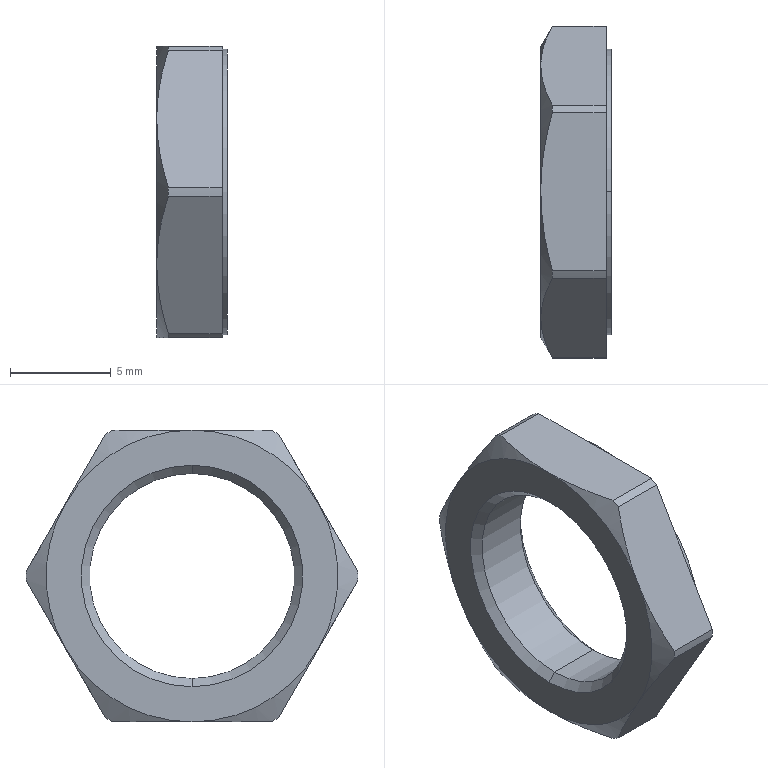Part | SolidWorks | features RefAxis 6, 3DProfileFeature 2, ICE 1, RevCut 1, Revolution 1, Scale 1 | 1 solid | 29 faces | box 3.5 x 16.5 x 14.5 mm | volume 336.894 mm3 | cone 10 | cylinder 10 | plane 9 | commonest cylinder face diameters 16.5 x6 10.188 x2 14.2 x2
STEP:
#1=CARTESIAN_POINT('',(4.831,0.00000041,-5.094));
#2=VERTEX_POINT('',#1);
#3=CARTESIAN_POINT('',(4.831,0.00000041,5.094));
#4=VERTEX_POINT('',#3);
#5=CARTESIAN_POINT('',(4.831,0.00000041,0.));
#6=DIRECTION('',(-1.,0.,0.));
#7=DIRECTION('',(0.,0.,1.));
#8=AXIS2_PLACEMENT_3D('',#5,#6,#7);
#9=CIRCLE('',#8,5.094);
#10=EDGE_CURVE('',#2,#4,#9,.T.);
#11=ORIENTED_EDGE('',*,*,#10,.T.);
#12=CARTESIAN_POINT('',(5.237,0.00000041,5.5));
#13=VERTEX_POINT('',#12);
#14=CARTESIAN_POINT('',(5.237,0.00000041,5.5));
#15=DIRECTION('',(0.7071,0.,0.7071));
#16=VECTOR('',#15,1000.);
#17=LINE('',#14,#16);
#18=EDGE_CURVE('',#4,#13,#17,.T.);
#19=ORIENTED_EDGE('',*,*,#18,.T.);
#20=CARTESIAN_POINT('',(5.237,0.00000041,-5.5));
#21=VERTEX_POINT('',#20);
#22=CARTESIAN_POINT('',(5.237,0.00000041,0.));
#23=DIRECTION('',(-1.,0.,0.));
#24=DIRECTION('',(0.,0.,1.));
#25=AXIS2_PLACEMENT_3D('',#22,#23,#24);
#26=CIRCLE('',#25,5.5);
#27=EDGE_CURVE('',#21,#13,#26,.T.);
#28=ORIENTED_EDGE('',*,*,#27,.F.);
#29=CARTESIAN_POINT('',(5.237,0.00000041,-5.5));
#30=DIRECTION('',(0.7071,0.,-0.7071));
#31=VECTOR('',#30,1000.);
#32=LINE('',#29,#31);
#33=EDGE_CURVE('',#2,#21,#32,.T.);
#34=ORIENTED_EDGE('',*,*,#33,.F.);
#35=EDGE_LOOP('',(#11,#19,#28,#34));
#36=FACE_OUTER_BOUND('',#35,.T.);
#37=CARTESIAN_POINT('',(5.237,0.00000041,0.));
#38=DIRECTION('',(1.,0.,0.));
#39=DIRECTION('',(0.,0.,-1.));
#40=AXIS2_PLACEMENT_3D('',#37,#38,#39);
#41=CONICAL_SURFACE('',#40,5.5,0.7854);
#42=ADVANCED_FACE('',(#36),#41,.F.);
#43=ORIENTED_EDGE('',*,*,#10,.F.);
#44=CARTESIAN_POINT('',(2.143,0.00000041,-5.094));
#45=VERTEX_POINT('',#44);
#46=CARTESIAN_POINT('',(5.237,0.00000041,-5.094));
#47=DIRECTION('',(-1.,0.,0.));
#48=VECTOR('',#47,1000.);
#49=LINE('',#46,#48);
#50=EDGE_CURVE('',#2,#45,#49,.T.);
#51=ORIENTED_EDGE('',*,*,#50,.T.);
#52=CARTESIAN_POINT('',(2.143,0.00000041,5.094));
#53=VERTEX_POINT('',#52);
#54=CARTESIAN_POINT('',(2.143,0.00000041,0.));
#55=DIRECTION('',(-1.,0.,0.));
#56=DIRECTION('',(0.,0.,1.));
#57=AXIS2_PLACEMENT_3D('',#54,#55,#56);
#58=CIRCLE('',#57,5.094);
#59=EDGE_CURVE('',#45,#53,#58,.T.);
#60=ORIENTED_EDGE('',*,*,#59,.T.);
#61=CARTESIAN_POINT('',(5.237,0.00000041,5.094));
#62=DIRECTION('',(-1.,0.,0.));
#63=VECTOR('',#62,1000.);
#64=LINE('',#61,#63);
#65=EDGE_CURVE('',#4,#53,#64,.T.);
#66=ORIENTED_EDGE('',*,*,#65,.F.);
#67=EDGE_LOOP('',(#43,#51,#60,#66));
#68=FACE_OUTER_BOUND('',#67,.T.);
#69=CARTESIAN_POINT('',(5.237,0.00000041,0.));
#70=DIRECTION('',(-1.,0.,0.));
#71=DIRECTION('',(0.,0.,1.));
#72=AXIS2_PLACEMENT_3D('',#69,#70,#71);
#73=CYLINDRICAL_SURFACE('',#72,5.094);
#74=ADVANCED_FACE('',(#68),#73,.F.);
#75=ORIENTED_EDGE('',*,*,#59,.F.);
#76=CARTESIAN_POINT('',(1.737,0.00000041,-5.5));
#77=VERTEX_POINT('',#76);
#78=CARTESIAN_POINT('',(2.143,0.00000041,-5.094));
#79=DIRECTION('',(-0.7071,0.,-0.7071));
#80=VECTOR('',#79,1000.);
#81=LINE('',#78,#80);
#82=EDGE_CURVE('',#45,#77,#81,.T.);
#83=ORIENTED_EDGE('',*,*,#82,.T.);
#84=CARTESIAN_POINT('',(1.737,0.00000041,5.5));
#85=VERTEX_POINT('',#84);
#86=CARTESIAN_POINT('',(1.737,0.00000041,0.));
#87=DIRECTION('',(-1.,0.,0.));
#88=DIRECTION('',(0.,0.,1.));
#89=AXIS2_PLACEMENT_3D('',#86,#87,#88);
#90=CIRCLE('',#89,5.5);
#91=EDGE_CURVE('',#77,#85,#90,.T.);
#92=ORIENTED_EDGE('',*,*,#91,.T.);
#93=CARTESIAN_POINT('',(2.143,0.00000041,5.094));
#94=DIRECTION('',(-0.7071,0.,0.7071));
#95=VECTOR('',#94,1000.);
#96=LINE('',#93,#95);
#97=EDGE_CURVE('',#53,#85,#96,.T.);
#98=ORIENTED_EDGE('',*,*,#97,.F.);
#99=EDGE_LOOP('',(#75,#83,#92,#98));
#100=FACE_OUTER_BOUND('',#99,.T.);
#101=CARTESIAN_POINT('',(2.143,0.00000041,0.));
#102=DIRECTION('',(-1.,0.,0.));
#103=DIRECTION('',(0.,0.,1.));
#104=AXIS2_PLACEMENT_3D('',#101,#102,#103);
#105=CONICAL_SURFACE('',#104,5.094,0.7854);
#106=ADVANCED_FACE('',(#100),#105,.F.);
#107=CARTESIAN_POINT('',(5.237,0.00000041,7.1));
#108=VERTEX_POINT('',#107);
#109=CARTESIAN_POINT('',(5.237,0.00000041,-7.1));
#110=VERTEX_POINT('',#109);
#111=CARTESIAN_POINT('',(5.237,0.00000041,0.));
#112=DIRECTION('',(-1.,0.,0.));
#113=DIRECTION('',(0.,0.,1.));
#114=AXIS2_PLACEMENT_3D('',#111,#112,#113);
#115=CIRCLE('',#114,7.1);
#116=EDGE_CURVE('',#108,#110,#115,.T.);
#117=ORIENTED_EDGE('',*,*,#116,.T.);
#118=CARTESIAN_POINT('',(4.987,0.00000041,-7.1));
#119=VERTEX_POINT('',#118);
#120=CARTESIAN_POINT('',(5.237,0.00000041,-7.1));
#121=DIRECTION('',(-1.,0.,0.));
#122=VECTOR('',#121,1000.);
#123=LINE('',#120,#122);
#124=EDGE_CURVE('',#110,#119,#123,.T.);
#125=ORIENTED_EDGE('',*,*,#124,.T.);
#126=CARTESIAN_POINT('',(4.987,0.00000041,7.1));
#127=VERTEX_POINT('',#126);
#128=CARTESIAN_POINT('',(4.987,0.00000041,0.));
#129=DIRECTION('',(-1.,0.,0.));
#130=DIRECTION('',(0.,0.,1.));
#131=AXIS2_PLACEMENT_3D('',#128,#129,#130);
#132=CIRCLE('',#131,7.1);
#133=EDGE_CURVE('',#127,#119,#132,.T.);
#134=ORIENTED_EDGE('',*,*,#133,.F.);
#135=CARTESIAN_POINT('',(5.237,0.00000041,7.1));
#136=DIRECTION('',(-1.,0.,0.));
#137=VECTOR('',#136,1000.);
#138=LINE('',#135,#137);
#139=EDGE_CURVE('',#108,#127,#138,.T.);
#140=ORIENTED_EDGE('',*,*,#139,.F.);
#141=EDGE_LOOP('',(#117,#125,#134,#140));
#142=FACE_OUTER_BOUND('',#141,.T.);
#143=CARTESIAN_POINT('',(5.237,0.00000041,0.));
#144=DIRECTION('',(-1.,0.,0.));
#145=DIRECTION('',(0.,0.,1.));
#146=AXIS2_PLACEMENT_3D('',#143,#144,#145);
#147=CYLINDRICAL_SURFACE('',#146,7.1);
#148=ADVANCED_FACE('',(#142),#147,.T.);
#149=CARTESIAN_POINT('',(2.314,-4.31,7.035));
#150=VERTEX_POINT('',#149);
#151=CARTESIAN_POINT('',(2.314,-3.937,7.25));
#152=VERTEX_POINT('',#151);
#153=CARTESIAN_POINT('',(2.314,0.00000041,0.));
#154=DIRECTION('',(-1.,0.,0.));
#155=DIRECTION('',(0.,0.,1.));
#156=AXIS2_PLACEMENT_3D('',#153,#154,#155);
#157=CIRCLE('',#156,8.25);
#158=EDGE_CURVE('',#150,#152,#157,.T.);
#159=ORIENTED_EDGE('',*,*,#158,.T.);
#160=CARTESIAN_POINT('',(1.737,0.00000041,7.25));
#161=VERTEX_POINT('',#160);
#162=CARTESIAN_POINT('',(2.314,-3.937,7.25));
#163=CARTESIAN_POINT('',(2.137,-3.295,7.25));
#164=CARTESIAN_POINT('',(1.99,-2.638,7.25));
#165=CARTESIAN_POINT('',(1.79,-1.325,7.25));
#166=CARTESIAN_POINT('',(1.737,-0.6643,7.25));
#167=CARTESIAN_POINT('',(1.737,0.00000041,7.25));
#168=B_SPLINE_CURVE_WITH_KNOTS('',3,(#162,#163,#164,#165,#166,#167),.UNSPECIFIED.,.F.,.F.,(4,2,4),(0.007715,0.009703,0.01169),.UNSPECIFIED.);
#169=EDGE_CURVE('',#152,#161,#168,.T.);
#170=ORIENTED_EDGE('',*,*,#169,.T.);
#171=CARTESIAN_POINT('',(1.737,-6.279,3.625));
#172=VERTEX_POINT('',#171);
#173=CARTESIAN_POINT('',(1.737,0.00000041,0.));
#174=DIRECTION('',(-1.,0.,0.));
#175=DIRECTION('',(0.,0.,1.));
#176=AXIS2_PLACEMENT_3D('',#173,#174,#175);
#177=CIRCLE('',#176,7.25);
#178=EDGE_CURVE('',#172,#161,#177,.T.);
#179=ORIENTED_EDGE('',*,*,#178,.F.);
#180=CARTESIAN_POINT('',(1.737,-6.279,3.625));
#181=CARTESIAN_POINT('',(1.737,-6.112,3.913));
#182=CARTESIAN_POINT('',(1.75,-5.945,4.203));
#183=CARTESIAN_POINT('',(1.803,-5.613,4.778));
#184=CARTESIAN_POINT('',(1.841,-5.448,5.064));
#185=CARTESIAN_POINT('',(1.992,-4.956,5.916));
#186=CARTESIAN_POINT('',(2.137,-4.632,6.477));
#187=CARTESIAN_POINT('',(2.314,-4.31,7.035));
#188=B_SPLINE_CURVE_WITH_KNOTS('',3,(#180,#181,#182,#183,#184,#185,#186,#187),.UNSPECIFIED.,.F.,.F.,(4,2,2,4),(0.003979,0.004968,0.005957,0.007936),.UNSPECIFIED.);
#189=EDGE_CURVE('',#172,#150,#188,.T.);
#190=ORIENTED_EDGE('',*,*,#189,.T.);
#191=EDGE_LOOP('',(#159,#170,#179,#190));
#192=FACE_OUTER_BOUND('',#191,.T.);
#193=CARTESIAN_POINT('',(2.314,0.00000041,0.));
#194=DIRECTION('',(1.,0.,0.));
#195=DIRECTION('',(0.,0.,-1.));
#196=AXIS2_PLACEMENT_3D('',#193,#194,#195);
#197=CONICAL_SURFACE('',#196,8.25,1.047);
#198=ADVANCED_FACE('',(#192),#197,.T.);
#199=CARTESIAN_POINT('',(2.314,-8.247,-0.2155));
#200=VERTEX_POINT('',#199);
#201=CARTESIAN_POINT('',(2.314,-8.247,0.2155));
#202=VERTEX_POINT('',#201);
#203=CARTESIAN_POINT('',(2.314,0.00000041,0.));
#204=DIRECTION('',(-1.,0.,0.));
#205=DIRECTION('',(0.,0.,1.));
#206=AXIS2_PLACEMENT_3D('',#203,#204,#205);
#207=CIRCLE('',#206,8.25);
#208=EDGE_CURVE('',#200,#202,#207,.T.);
#209=ORIENTED_EDGE('',*,*,#208,.T.);
#210=CARTESIAN_POINT('',(2.314,-8.247,0.2155));
#211=CARTESIAN_POINT('',(2.136,-7.924,0.7746));
#212=CARTESIAN_POINT('',(1.991,-7.599,1.337));
#213=CARTESIAN_POINT('',(1.791,-6.944,2.473));
#214=CARTESIAN_POINT('',(1.737,-6.613,3.046));
#215=CARTESIAN_POINT('',(1.737,-6.279,3.625));
#216=B_SPLINE_CURVE_WITH_KNOTS('',3,(#210,#211,#212,#213,#214,#215),.UNSPECIFIED.,.F.,.F.,(4,2,4),(0.000000373,0.00199,0.003979),.UNSPECIFIED.);
#217=EDGE_CURVE('',#202,#172,#216,.T.);
#218=ORIENTED_EDGE('',*,*,#217,.T.);
#219=CARTESIAN_POINT('',(1.737,-6.279,-3.625));
#220=VERTEX_POINT('',#219);
#221=CARTESIAN_POINT('',(1.737,0.00000041,0.));
#222=DIRECTION('',(-1.,0.,0.));
#223=DIRECTION('',(0.,0.,1.));
#224=AXIS2_PLACEMENT_3D('',#221,#222,#223);
#225=CIRCLE('',#224,7.25);
#226=EDGE_CURVE('',#220,#172,#225,.T.);
#227=ORIENTED_EDGE('',*,*,#226,.F.);
#228=CARTESIAN_POINT('',(1.737,-6.279,-3.625));
#229=CARTESIAN_POINT('',(1.737,-6.445,-3.337));
#230=CARTESIAN_POINT('',(1.75,-6.612,-3.047));
#231=CARTESIAN_POINT('',(1.803,-6.944,-2.472));
#232=CARTESIAN_POINT('',(1.841,-7.109,-2.186));
#233=CARTESIAN_POINT('',(1.992,-7.601,-1.334));
#234=CARTESIAN_POINT('',(2.137,-7.926,-0.7726));
#235=CARTESIAN_POINT('',(2.314,-8.247,-0.2155));
#236=B_SPLINE_CURVE_WITH_KNOTS('',3,(#228,#229,#230,#231,#232,#233,#234,#235),.UNSPECIFIED.,.F.,.F.,(4,2,2,4),(0.003979,0.004968,0.005957,0.007936),.UNSPECIFIED.);
#237=EDGE_CURVE('',#220,#200,#236,.T.);
#238=ORIENTED_EDGE('',*,*,#237,.T.);
#239=EDGE_LOOP('',(#209,#218,#227,#238));
#240=FACE_OUTER_BOUND('',#239,.T.);
#241=CARTESIAN_POINT('',(2.314,0.00000041,0.));
#242=DIRECTION('',(1.,0.,0.));
#243=DIRECTION('',(0.,0.,-1.));
#244=AXIS2_PLACEMENT_3D('',#241,#242,#243);
#245=CONICAL_SURFACE('',#244,8.25,1.047);
#246=ADVANCED_FACE('',(#240),#245,.T.);
#247=CARTESIAN_POINT('',(2.314,-3.937,-7.25));
#248=VERTEX_POINT('',#247);
#249=CARTESIAN_POINT('',(2.314,-4.31,-7.035));
#250=VERTEX_POINT('',#249);
#251=CARTESIAN_POINT('',(2.314,0.00000041,0.));
#252=DIRECTION('',(-1.,0.,0.));
#253=DIRECTION('',(0.,0.,1.));
#254=AXIS2_PLACEMENT_3D('',#251,#252,#253);
#255=CIRCLE('',#254,8.25);
#256=EDGE_CURVE('',#248,#250,#255,.T.);
#257=ORIENTED_EDGE('',*,*,#256,.T.);
#258=CARTESIAN_POINT('',(2.314,-4.31,-7.035));
#259=CARTESIAN_POINT('',(2.136,-4.633,-6.475));
#260=CARTESIAN_POINT('',(1.991,-4.958,-5.913));
#261=CARTESIAN_POINT('',(1.791,-5.614,-4.777));
#262=CARTESIAN_POINT('',(1.737,-5.944,-4.204));
#263=CARTESIAN_POINT('',(1.737,-6.279,-3.625));
#264=B_SPLINE_CURVE_WITH_KNOTS('',3,(#258,#259,#260,#261,#262,#263),.UNSPECIFIED.,.F.,.F.,(4,2,4),(0.000000373,0.00199,0.003979),.UNSPECIFIED.);
#265=EDGE_CURVE('',#250,#220,#264,.T.);
#266=ORIENTED_EDGE('',*,*,#265,.T.);
#267=CARTESIAN_POINT('',(1.737,0.00000041,-7.25));
#268=VERTEX_POINT('',#267);
#269=CARTESIAN_POINT('',(1.737,0.00000041,0.));
#270=DIRECTION('',(-1.,0.,0.));
#271=DIRECTION('',(0.,0.,1.));
#272=AXIS2_PLACEMENT_3D('',#269,#270,#271);
#273=CIRCLE('',#272,7.25);
#274=EDGE_CURVE('',#268,#220,#273,.T.);
#275=ORIENTED_EDGE('',*,*,#274,.F.);
#276=CARTESIAN_POINT('',(1.737,0.00000041,-7.25));
#277=CARTESIAN_POINT('',(1.737,-0.6643,-7.25));
#278=CARTESIAN_POINT('',(1.79,-1.325,-7.25));
#279=CARTESIAN_POINT('',(1.99,-2.638,-7.25));
#280=CARTESIAN_POINT('',(2.137,-3.295,-7.25));
#281=CARTESIAN_POINT('',(2.314,-3.937,-7.25));
#282=B_SPLINE_CURVE_WITH_KNOTS('',3,(#276,#277,#278,#279,#280,#281),.UNSPECIFIED.,.F.,.F.,(4,2,4),(0.007306,0.00929,0.01127),.UNSPECIFIED.);
#283=EDGE_CURVE('',#268,#248,#282,.T.);
#284=ORIENTED_EDGE('',*,*,#283,.T.);
#285=EDGE_LOOP('',(#257,#266,#275,#284));
#286=FACE_OUTER_BOUND('',#285,.T.);
#287=CARTESIAN_POINT('',(2.314,0.00000041,0.));
#288=DIRECTION('',(1.,0.,0.));
#289=DIRECTION('',(0.,0.,-1.));
#290=AXIS2_PLACEMENT_3D('',#287,#288,#289);
#291=CONICAL_SURFACE('',#290,8.25,1.047);
#292=ADVANCED_FACE('',(#286),#291,.T.);
#293=CARTESIAN_POINT('',(2.314,4.31,-7.035));
#294=VERTEX_POINT('',#293);
#295=CARTESIAN_POINT('',(2.314,3.937,-7.25));
#296=VERTEX_POINT('',#295);
#297=CARTESIAN_POINT('',(2.314,0.00000041,0.));
#298=DIRECTION('',(-1.,0.,0.));
#299=DIRECTION('',(0.,0.,1.));
#300=AXIS2_PLACEMENT_3D('',#297,#298,#299);
#301=CIRCLE('',#300,8.25);
#302=EDGE_CURVE('',#294,#296,#301,.T.);
#303=ORIENTED_EDGE('',*,*,#302,.T.);
#304=CARTESIAN_POINT('',(2.314,3.937,-7.25));
#305=CARTESIAN_POINT('',(2.139,3.299,-7.25));
#306=CARTESIAN_POINT('',(1.993,2.654,-7.25));
#307=CARTESIAN_POINT('',(1.792,1.338,-7.25));
#308=CARTESIAN_POINT('',(1.737,0.6644,-7.25));
#309=CARTESIAN_POINT('',(1.737,0.00000041,-7.25));
#310=B_SPLINE_CURVE_WITH_KNOTS('',3,(#304,#305,#306,#307,#308,#309),.UNSPECIFIED.,.F.,.F.,(4,2,4),(0.003338,0.005322,0.007306),.UNSPECIFIED.);
#311=EDGE_CURVE('',#296,#268,#310,.T.);
#312=ORIENTED_EDGE('',*,*,#311,.T.);
#313=CARTESIAN_POINT('',(1.737,6.279,-3.625));
#314=VERTEX_POINT('',#313);
#315=CARTESIAN_POINT('',(1.737,0.00000041,0.));
#316=DIRECTION('',(-1.,0.,0.));
#317=DIRECTION('',(0.,0.,1.));
#318=AXIS2_PLACEMENT_3D('',#315,#316,#317);
#319=CIRCLE('',#318,7.25);
#320=EDGE_CURVE('',#314,#268,#319,.T.);
#321=ORIENTED_EDGE('',*,*,#320,.F.);
#322=CARTESIAN_POINT('',(1.737,6.279,-3.625));
#323=CARTESIAN_POINT('',(1.737,6.112,-3.913));
#324=CARTESIAN_POINT('',(1.75,5.945,-4.203));
#325=CARTESIAN_POINT('',(1.803,5.613,-4.778));
#326=CARTESIAN_POINT('',(1.841,5.448,-5.064));
#327=CARTESIAN_POINT('',(1.992,4.956,-5.916));
#328=CARTESIAN_POINT('',(2.137,4.632,-6.477));
#329=CARTESIAN_POINT('',(2.314,4.31,-7.035));
#330=B_SPLINE_CURVE_WITH_KNOTS('',3,(#322,#323,#324,#325,#326,#327,#328,#329),.UNSPECIFIED.,.F.,.F.,(4,2,2,4),(0.003979,0.004968,0.005957,0.007936),.UNSPECIFIED.);
#331=EDGE_CURVE('',#314,#294,#330,.T.);
#332=ORIENTED_EDGE('',*,*,#331,.T.);
#333=EDGE_LOOP('',(#303,#312,#321,#332));
#334=FACE_OUTER_BOUND('',#333,.T.);
#335=CARTESIAN_POINT('',(2.314,0.00000041,0.));
#336=DIRECTION('',(1.,0.,0.));
#337=DIRECTION('',(0.,0.,-1.));
#338=AXIS2_PLACEMENT_3D('',#335,#336,#337);
#339=CONICAL_SURFACE('',#338,8.25,1.047);
#340=ADVANCED_FACE('',(#334),#339,.T.);
#341=CARTESIAN_POINT('',(2.314,8.247,0.2155));
#342=VERTEX_POINT('',#341);
#343=CARTESIAN_POINT('',(2.314,8.247,-0.2155));
#344=VERTEX_POINT('',#343);
#345=CARTESIAN_POINT('',(2.314,0.00000041,0.));
#346=DIRECTION('',(-1.,0.,0.));
#347=DIRECTION('',(0.,0.,1.));
#348=AXIS2_PLACEMENT_3D('',#345,#346,#347);
#349=CIRCLE('',#348,8.25);
#350=EDGE_CURVE('',#342,#344,#349,.T.);
#351=ORIENTED_EDGE('',*,*,#350,.T.);
#352=CARTESIAN_POINT('',(2.314,8.247,-0.2155));
#353=CARTESIAN_POINT('',(2.136,7.924,-0.7746));
#354=CARTESIAN_POINT('',(1.991,7.599,-1.337));
#355=CARTESIAN_POINT('',(1.791,6.944,-2.473));
#356=CARTESIAN_POINT('',(1.737,6.613,-3.046));
#357=CARTESIAN_POINT('',(1.737,6.279,-3.625));
#358=B_SPLINE_CURVE_WITH_KNOTS('',3,(#352,#353,#354,#355,#356,#357),.UNSPECIFIED.,.F.,.F.,(4,2,4),(0.000000373,0.00199,0.003979),.UNSPECIFIED.);
#359=EDGE_CURVE('',#344,#314,#358,.T.);
#360=ORIENTED_EDGE('',*,*,#359,.T.);
#361=CARTESIAN_POINT('',(1.737,6.279,3.625));
#362=VERTEX_POINT('',#361);
#363=CARTESIAN_POINT('',(1.737,0.00000041,0.));
#364=DIRECTION('',(-1.,0.,0.));
#365=DIRECTION('',(0.,0.,1.));
#366=AXIS2_PLACEMENT_3D('',#363,#364,#365);
#367=CIRCLE('',#366,7.25);
#368=EDGE_CURVE('',#362,#314,#367,.T.);
#369=ORIENTED_EDGE('',*,*,#368,.F.);
#370=CARTESIAN_POINT('',(1.737,6.279,3.625));
#371=CARTESIAN_POINT('',(1.737,6.445,3.337));
#372=CARTESIAN_POINT('',(1.75,6.612,3.047));
#373=CARTESIAN_POINT('',(1.803,6.944,2.472));
#374=CARTESIAN_POINT('',(1.841,7.109,2.186));
#375=CARTESIAN_POINT('',(1.992,7.601,1.334));
#376=CARTESIAN_POINT('',(2.137,7.926,0.7726));
#377=CARTESIAN_POINT('',(2.314,8.247,0.2155));
#378=B_SPLINE_CURVE_WITH_KNOTS('',3,(#370,#371,#372,#373,#374,#375,#376,#377),.UNSPECIFIED.,.F.,.F.,(4,2,2,4),(0.003979,0.004968,0.005957,0.007936),.UNSPECIFIED.);
#379=EDGE_CURVE('',#362,#342,#378,.T.);
#380=ORIENTED_EDGE('',*,*,#379,.T.);
#381=EDGE_LOOP('',(#351,#360,#369,#380));
#382=FACE_OUTER_BOUND('',#381,.T.);
#383=CARTESIAN_POINT('',(2.314,0.00000041,0.));
#384=DIRECTION('',(1.,0.,0.));
#385=DIRECTION('',(0.,0.,-1.));
#386=AXIS2_PLACEMENT_3D('',#383,#384,#385);
#387=CONICAL_SURFACE('',#386,8.25,1.047);
#388=ADVANCED_FACE('',(#382),#387,.T.);
#389=CARTESIAN_POINT('',(4.987,-4.31,7.035));
#390=VERTEX_POINT('',#389);
#391=CARTESIAN_POINT('',(4.987,-3.937,7.25));
#392=VERTEX_POINT('',#391);
#393=CARTESIAN_POINT('',(4.987,0.00000041,0.));
#394=DIRECTION('',(-1.,0.,0.));
#395=DIRECTION('',(0.,0.,1.));
#396=AXIS2_PLACEMENT_3D('',#393,#394,#395);
#397=CIRCLE('',#396,8.25);
#398=EDGE_CURVE('',#390,#392,#397,.T.);
#399=ORIENTED_EDGE('',*,*,#398,.T.);
#400=CARTESIAN_POINT('',(5.237,-3.937,7.25));
#401=DIRECTION('',(-1.,0.,0.));
#402=VECTOR('',#401,1000.);
#403=LINE('',#400,#402);
#404=EDGE_CURVE('',#392,#152,#403,.T.);
#405=ORIENTED_EDGE('',*,*,#404,.T.);
#406=ORIENTED_EDGE('',*,*,#158,.F.);
#407=CARTESIAN_POINT('',(5.237,-4.31,7.035));
#408=DIRECTION('',(1.,0.,0.));
#409=VECTOR('',#408,1000.);
#410=LINE('',#407,#409);
#411=EDGE_CURVE('',#150,#390,#410,.T.);
#412=ORIENTED_EDGE('',*,*,#411,.T.);
#413=EDGE_LOOP('',(#399,#405,#406,#412));
#414=FACE_OUTER_BOUND('',#413,.T.);
#415=CARTESIAN_POINT('',(5.237,0.00000041,0.));
#416=DIRECTION('',(-1.,0.,0.));
#417=DIRECTION('',(0.,0.,1.));
#418=AXIS2_PLACEMENT_3D('',#415,#416,#417);
#419=CYLINDRICAL_SURFACE('',#418,8.25);
#420=ADVANCED_FACE('',(#414),#419,.T.);
#421=CARTESIAN_POINT('',(4.987,-8.247,-0.2155));
#422=VERTEX_POINT('',#421);
#423=CARTESIAN_POINT('',(4.987,-8.247,0.2155));
#424=VERTEX_POINT('',#423);
#425=CARTESIAN_POINT('',(4.987,0.00000041,0.));
#426=DIRECTION('',(-1.,0.,0.));
#427=DIRECTION('',(0.,0.,1.));
#428=AXIS2_PLACEMENT_3D('',#425,#426,#427);
#429=CIRCLE('',#428,8.25);
#430=EDGE_CURVE('',#422,#424,#429,.T.);
#431=ORIENTED_EDGE('',*,*,#430,.T.);
#432=CARTESIAN_POINT('',(5.237,-8.247,0.2155));
#433=DIRECTION('',(-1.,0.,0.));
#434=VECTOR('',#433,1000.);
#435=LINE('',#432,#434);
#436=EDGE_CURVE('',#424,#202,#435,.T.);
#437=ORIENTED_EDGE('',*,*,#436,.T.);
#438=ORIENTED_EDGE('',*,*,#208,.F.);
#439=CARTESIAN_POINT('',(5.237,-8.247,-0.2155));
#440=DIRECTION('',(1.,0.,0.));
#441=VECTOR('',#440,1000.);
#442=LINE('',#439,#441);
#443=EDGE_CURVE('',#200,#422,#442,.T.);
#444=ORIENTED_EDGE('',*,*,#443,.T.);
#445=EDGE_LOOP('',(#431,#437,#438,#444));
#446=FACE_OUTER_BOUND('',#445,.T.);
#447=CARTESIAN_POINT('',(5.237,0.00000041,0.));
#448=DIRECTION('',(-1.,0.,0.));
#449=DIRECTION('',(0.,0.,1.));
#450=AXIS2_PLACEMENT_3D('',#447,#448,#449);
#451=CYLINDRICAL_SURFACE('',#450,8.25);
#452=ADVANCED_FACE('',(#446),#451,.T.);
#453=CARTESIAN_POINT('',(4.987,-3.937,-7.25));
#454=VERTEX_POINT('',#453);
#455=CARTESIAN_POINT('',(4.987,-4.31,-7.035));
#456=VERTEX_POINT('',#455);
#457=CARTESIAN_POINT('',(4.987,0.00000041,0.));
#458=DIRECTION('',(-1.,0.,0.));
#459=DIRECTION('',(0.,0.,1.));
#460=AXIS2_PLACEMENT_3D('',#457,#458,#459);
#461=CIRCLE('',#460,8.25);
#462=EDGE_CURVE('',#454,#456,#461,.T.);
#463=ORIENTED_EDGE('',*,*,#462,.T.);
#464=CARTESIAN_POINT('',(5.237,-4.31,-7.035));
#465=DIRECTION('',(-1.,0.,0.));
#466=VECTOR('',#465,1000.);
#467=LINE('',#464,#466);
#468=EDGE_CURVE('',#456,#250,#467,.T.);
#469=ORIENTED_EDGE('',*,*,#468,.T.);
#470=ORIENTED_EDGE('',*,*,#256,.F.);
#471=CARTESIAN_POINT('',(5.237,-3.937,-7.25));
#472=DIRECTION('',(1.,0.,0.));
#473=VECTOR('',#472,1000.);
#474=LINE('',#471,#473);
#475=EDGE_CURVE('',#248,#454,#474,.T.);
#476=ORIENTED_EDGE('',*,*,#475,.T.);
#477=EDGE_LOOP('',(#463,#469,#470,#476));
#478=FACE_OUTER_BOUND('',#477,.T.);
#479=CARTESIAN_POINT('',(5.237,0.00000041,0.));
#480=DIRECTION('',(-1.,0.,0.));
#481=DIRECTION('',(0.,0.,1.));
#482=AXIS2_PLACEMENT_3D('',#479,#480,#481);
#483=CYLINDRICAL_SURFACE('',#482,8.25);
#484=ADVANCED_FACE('',(#478),#483,.T.);
#485=CARTESIAN_POINT('',(4.987,4.31,-7.035));
#486=VERTEX_POINT('',#485);
#487=CARTESIAN_POINT('',(4.987,3.937,-7.25));
#488=VERTEX_POINT('',#487);
#489=CARTESIAN_POINT('',(4.987,0.00000041,0.));
#490=DIRECTION('',(-1.,0.,0.));
#491=DIRECTION('',(0.,0.,1.));
#492=AXIS2_PLACEMENT_3D('',#489,#490,#491);
#493=CIRCLE('',#492,8.25);
#494=EDGE_CURVE('',#486,#488,#493,.T.);
#495=ORIENTED_EDGE('',*,*,#494,.T.);
#496=CARTESIAN_POINT('',(5.237,3.937,-7.25));
#497=DIRECTION('',(-1.,0.,0.));
#498=VECTOR('',#497,1000.);
#499=LINE('',#496,#498);
#500=EDGE_CURVE('',#488,#296,#499,.T.);
#501=ORIENTED_EDGE('',*,*,#500,.T.);
#502=ORIENTED_EDGE('',*,*,#302,.F.);
#503=CARTESIAN_POINT('',(5.237,4.31,-7.035));
#504=DIRECTION('',(1.,0.,0.));
#505=VECTOR('',#504,1000.);
#506=LINE('',#503,#505);
#507=EDGE_CURVE('',#294,#486,#506,.T.);
#508=ORIENTED_EDGE('',*,*,#507,.T.);
#509=EDGE_LOOP('',(#495,#501,#502,#508));
#510=FACE_OUTER_BOUND('',#509,.T.);
#511=CARTESIAN_POINT('',(5.237,0.00000041,0.));
#512=DIRECTION('',(-1.,0.,0.));
#513=DIRECTION('',(0.,0.,1.));
#514=AXIS2_PLACEMENT_3D('',#511,#512,#513);
#515=CYLINDRICAL_SURFACE('',#514,8.25);
#516=ADVANCED_FACE('',(#510),#515,.T.);
#517=CARTESIAN_POINT('',(4.987,8.247,0.2155));
#518=VERTEX_POINT('',#517);
#519=CARTESIAN_POINT('',(4.987,8.247,-0.2155));
#520=VERTEX_POINT('',#519);
#521=CARTESIAN_POINT('',(4.987,0.00000041,0.));
#522=DIRECTION('',(-1.,0.,0.));
#523=DIRECTION('',(0.,0.,1.));
#524=AXIS2_PLACEMENT_3D('',#521,#522,#523);
#525=CIRCLE('',#524,8.25);
#526=EDGE_CURVE('',#518,#520,#525,.T.);
#527=ORIENTED_EDGE('',*,*,#526,.T.);
#528=CARTESIAN_POINT('',(5.237,8.247,-0.2155));
#529=DIRECTION('',(-1.,0.,0.));
#530=VECTOR('',#529,1000.);
#531=LINE('',#528,#530);
#532=EDGE_CURVE('',#520,#344,#531,.T.);
#533=ORIENTED_EDGE('',*,*,#532,.T.);
#534=ORIENTED_EDGE('',*,*,#350,.F.);
#535=CARTESIAN_POINT('',(5.237,8.247,0.2155));
#536=DIRECTION('',(1.,0.,0.));
#537=VECTOR('',#536,1000.);
#538=LINE('',#535,#537);
#539=EDGE_CURVE('',#342,#518,#538,.T.);
#540=ORIENTED_EDGE('',*,*,#539,.T.);
#541=EDGE_LOOP('',(#527,#533,#534,#540));
#542=FACE_OUTER_BOUND('',#541,.T.);
#543=CARTESIAN_POINT('',(5.237,0.00000041,0.));
#544=DIRECTION('',(-1.,0.,0.));
#545=DIRECTION('',(0.,0.,1.));
#546=AXIS2_PLACEMENT_3D('',#543,#544,#545);
#547=CYLINDRICAL_SURFACE('',#546,8.25);
#548=ADVANCED_FACE('',(#542),#547,.T.);
#549=CARTESIAN_POINT('',(1.737,0.00000041,0.));
#550=DIRECTION('',(-1.,0.,0.));
#551=DIRECTION('',(0.,0.,1.));
#552=AXIS2_PLACEMENT_3D('',#549,#550,#551);
#553=CIRCLE('',#552,5.5);
#554=EDGE_CURVE('',#85,#77,#553,.T.);
#555=ORIENTED_EDGE('',*,*,#554,.F.);
#556=ORIENTED_EDGE('',*,*,#91,.F.);
#557=EDGE_LOOP('',(#555,#556));
#558=FACE_BOUND('',#557,.T.);
#559=CARTESIAN_POINT('',(1.737,0.00000041,0.));
#560=DIRECTION('',(-1.,0.,0.));
#561=DIRECTION('',(0.,0.,1.));
#562=AXIS2_PLACEMENT_3D('',#559,#560,#561);
#563=CIRCLE('',#562,7.25);
#564=EDGE_CURVE('',#161,#362,#563,.T.);
#565=ORIENTED_EDGE('',*,*,#564,.T.);
#566=ORIENTED_EDGE('',*,*,#368,.T.);
#567=ORIENTED_EDGE('',*,*,#320,.T.);
#568=ORIENTED_EDGE('',*,*,#274,.T.);
#569=ORIENTED_EDGE('',*,*,#226,.T.);
#570=ORIENTED_EDGE('',*,*,#178,.T.);
#571=EDGE_LOOP('',(#565,#566,#567,#568,#569,#570));
#572=FACE_OUTER_BOUND('',#571,.T.);
#573=CARTESIAN_POINT('',(1.737,0.00000041,0.));
#574=DIRECTION('',(1.,0.,0.));
#575=DIRECTION('',(0.,0.,-1.));
#576=AXIS2_PLACEMENT_3D('',#573,#574,#575);
#577=PLANE('',#576);
#578=ADVANCED_FACE('',(#558,#572),#577,.F.);
#579=ORIENTED_EDGE('',*,*,#564,.F.);
#580=CARTESIAN_POINT('',(2.314,3.937,7.25));
#581=VERTEX_POINT('',#580);
#582=CARTESIAN_POINT('',(1.737,0.00000041,7.25));
#583=CARTESIAN_POINT('',(1.737,0.6644,7.25));
#584=CARTESIAN_POINT('',(1.792,1.338,7.25));
#585=CARTESIAN_POINT('',(1.993,2.654,7.25));
#586=CARTESIAN_POINT('',(2.139,3.299,7.25));
#587=CARTESIAN_POINT('',(2.314,3.937,7.25));
#588=B_SPLINE_CURVE_WITH_KNOTS('',3,(#582,#583,#584,#585,#586,#587),.UNSPECIFIED.,.F.,.F.,(4,2,4),(0.01169,0.01368,0.01567),.UNSPECIFIED.);
#589=EDGE_CURVE('',#161,#581,#588,.T.);
#590=ORIENTED_EDGE('',*,*,#589,.T.);
#591=CARTESIAN_POINT('',(2.314,4.31,7.035));
#592=VERTEX_POINT('',#591);
#593=CARTESIAN_POINT('',(2.314,0.00000041,0.));
#594=DIRECTION('',(-1.,0.,0.));
#595=DIRECTION('',(0.,0.,1.));
#596=AXIS2_PLACEMENT_3D('',#593,#594,#595);
#597=CIRCLE('',#596,8.25);
#598=EDGE_CURVE('',#581,#592,#597,.T.);
#599=ORIENTED_EDGE('',*,*,#598,.T.);
#600=CARTESIAN_POINT('',(2.314,4.31,7.035));
#601=CARTESIAN_POINT('',(2.136,4.633,6.475));
#602=CARTESIAN_POINT('',(1.991,4.958,5.913));
#603=CARTESIAN_POINT('',(1.791,5.614,4.777));
#604=CARTESIAN_POINT('',(1.737,5.944,4.204));
#605=CARTESIAN_POINT('',(1.737,6.279,3.625));
#606=B_SPLINE_CURVE_WITH_KNOTS('',3,(#600,#601,#602,#603,#604,#605),.UNSPECIFIED.,.F.,.F.,(4,2,4),(0.000000373,0.00199,0.003979),.UNSPECIFIED.);
#607=EDGE_CURVE('',#592,#362,#606,.T.);
#608=ORIENTED_EDGE('',*,*,#607,.T.);
#609=EDGE_LOOP('',(#579,#590,#599,#608));
#610=FACE_OUTER_BOUND('',#609,.T.);
#611=CARTESIAN_POINT('',(2.314,0.00000041,0.));
#612=DIRECTION('',(1.,0.,0.));
#613=DIRECTION('',(0.,0.,-1.));
#614=AXIS2_PLACEMENT_3D('',#611,#612,#613);
#615=CONICAL_SURFACE('',#614,8.25,1.047);
#616=ADVANCED_FACE('',(#610),#615,.T.);
#617=ORIENTED_EDGE('',*,*,#598,.F.);
#618=CARTESIAN_POINT('',(4.987,3.937,7.25));
#619=VERTEX_POINT('',#618);
#620=CARTESIAN_POINT('',(5.237,3.937,7.25));
#621=DIRECTION('',(1.,0.,0.));
#622=VECTOR('',#621,1000.);
#623=LINE('',#620,#622);
#624=EDGE_CURVE('',#581,#619,#623,.T.);
#625=ORIENTED_EDGE('',*,*,#624,.T.);
#626=CARTESIAN_POINT('',(4.987,4.31,7.035));
#627=VERTEX_POINT('',#626);
#628=CARTESIAN_POINT('',(4.987,0.00000041,0.));
#629=DIRECTION('',(-1.,0.,0.));
#630=DIRECTION('',(0.,0.,1.));
#631=AXIS2_PLACEMENT_3D('',#628,#629,#630);
#632=CIRCLE('',#631,8.25);
#633=EDGE_CURVE('',#619,#627,#632,.T.);
#634=ORIENTED_EDGE('',*,*,#633,.T.);
#635=CARTESIAN_POINT('',(5.237,4.31,7.035));
#636=DIRECTION('',(-1.,0.,0.));
#637=VECTOR('',#636,1000.);
#638=LINE('',#635,#637);
#639=EDGE_CURVE('',#627,#592,#638,.T.);
#640=ORIENTED_EDGE('',*,*,#639,.T.);
#641=EDGE_LOOP('',(#617,#625,#634,#640));
#642=FACE_OUTER_BOUND('',#641,.T.);
#643=CARTESIAN_POINT('',(5.237,0.00000041,0.));
#644=DIRECTION('',(-1.,0.,0.));
#645=DIRECTION('',(0.,0.,1.));
#646=AXIS2_PLACEMENT_3D('',#643,#644,#645);
#647=CYLINDRICAL_SURFACE('',#646,8.25);
#648=ADVANCED_FACE('',(#642),#647,.T.);
#649=ORIENTED_EDGE('',*,*,#633,.F.);
#650=CARTESIAN_POINT('',(4.987,8.25,7.25));
#651=DIRECTION('',(0.,-1.,0.));
#652=VECTOR('',#651,1000.);
#653=LINE('',#650,#652);
#654=EDGE_CURVE('',#619,#392,#653,.T.);
#655=ORIENTED_EDGE('',*,*,#654,.T.);
#656=ORIENTED_EDGE('',*,*,#398,.F.);
#657=CARTESIAN_POINT('',(4.987,-4.216,7.197));
#658=DIRECTION('',(0.,-0.5,-0.866));
#659=VECTOR('',#658,1000.);
#660=LINE('',#657,#659);
#661=EDGE_CURVE('',#390,#424,#660,.T.);
#662=ORIENTED_EDGE('',*,*,#661,.T.);
#663=ORIENTED_EDGE('',*,*,#430,.F.);
#664=CARTESIAN_POINT('',(4.987,-4.216,-7.197));
#665=DIRECTION('',(0.,0.5,-0.866));
#666=VECTOR('',#665,1000.);
#667=LINE('',#664,#666);
#668=EDGE_CURVE('',#422,#456,#667,.T.);
#669=ORIENTED_EDGE('',*,*,#668,.T.);
#670=ORIENTED_EDGE('',*,*,#462,.F.);
#671=CARTESIAN_POINT('',(4.987,8.25,-7.25));
#672=DIRECTION('',(0.,1.,0.));
#673=VECTOR('',#672,1000.);
#674=LINE('',#671,#673);
#675=EDGE_CURVE('',#454,#488,#674,.T.);
#676=ORIENTED_EDGE('',*,*,#675,.T.);
#677=ORIENTED_EDGE('',*,*,#494,.F.);
#678=CARTESIAN_POINT('',(4.987,8.341,-0.05265));
#679=DIRECTION('',(0.,0.5,0.866));
#680=VECTOR('',#679,1000.);
#681=LINE('',#678,#680);
#682=EDGE_CURVE('',#486,#520,#681,.T.);
#683=ORIENTED_EDGE('',*,*,#682,.T.);
#684=ORIENTED_EDGE('',*,*,#526,.F.);
#685=CARTESIAN_POINT('',(4.987,8.341,0.05265));
#686=DIRECTION('',(0.,-0.5,0.866));
#687=VECTOR('',#686,1000.);
#688=LINE('',#685,#687);
#689=EDGE_CURVE('',#518,#627,#688,.T.);
#690=ORIENTED_EDGE('',*,*,#689,.T.);
#691=EDGE_LOOP('',(#649,#655,#656,#662,#663,#669,#670,#676,#677,#683,#684,#690));
#692=FACE_OUTER_BOUND('',#691,.T.);
#693=ORIENTED_EDGE('',*,*,#133,.T.);
#694=CARTESIAN_POINT('',(4.987,0.00000041,0.));
#695=DIRECTION('',(-1.,0.,0.));
#696=DIRECTION('',(0.,0.,1.));
#697=AXIS2_PLACEMENT_3D('',#694,#695,#696);
#698=CIRCLE('',#697,7.1);
#699=EDGE_CURVE('',#119,#127,#698,.T.);
#700=ORIENTED_EDGE('',*,*,#699,.T.);
#701=EDGE_LOOP('',(#693,#700));
#702=FACE_BOUND('',#701,.T.);
#703=CARTESIAN_POINT('',(4.987,8.25,0.));
#704=DIRECTION('',(-1.,0.,0.));
#705=DIRECTION('',(0.,0.,1.));
#706=AXIS2_PLACEMENT_3D('',#703,#704,#705);
#707=PLANE('',#706);
#708=ADVANCED_FACE('',(#692,#702),#707,.F.);
#709=ORIENTED_EDGE('',*,*,#124,.F.);
#710=CARTESIAN_POINT('',(5.237,0.00000041,0.));
#711=DIRECTION('',(-1.,0.,0.));
#712=DIRECTION('',(0.,0.,1.));
#713=AXIS2_PLACEMENT_3D('',#710,#711,#712);
#714=CIRCLE('',#713,7.1);
#715=EDGE_CURVE('',#110,#108,#714,.T.);
#716=ORIENTED_EDGE('',*,*,#715,.T.);
#717=ORIENTED_EDGE('',*,*,#139,.T.);
#718=ORIENTED_EDGE('',*,*,#699,.F.);
#719=EDGE_LOOP('',(#709,#716,#717,#718));
#720=FACE_OUTER_BOUND('',#719,.T.);
#721=CARTESIAN_POINT('',(5.237,0.00000041,0.));
#722=DIRECTION('',(-1.,0.,0.));
#723=DIRECTION('',(0.,0.,1.));
#724=AXIS2_PLACEMENT_3D('',#721,#722,#723);
#725=CYLINDRICAL_SURFACE('',#724,7.1);
#726=ADVANCED_FACE('',(#720),#725,.T.);
#727=ORIENTED_EDGE('',*,*,#27,.T.);
#728=CARTESIAN_POINT('',(5.237,0.00000041,0.));
#729=DIRECTION('',(-1.,0.,0.));
#730=DIRECTION('',(0.,0.,1.));
#731=AXIS2_PLACEMENT_3D('',#728,#729,#730);
#732=CIRCLE('',#731,5.5);
#733=EDGE_CURVE('',#13,#21,#732,.T.);
#734=ORIENTED_EDGE('',*,*,#733,.T.);
#735=EDGE_LOOP('',(#727,#734));
#736=FACE_BOUND('',#735,.T.);
#737=ORIENTED_EDGE('',*,*,#116,.F.);
#738=ORIENTED_EDGE('',*,*,#715,.F.);
#739=EDGE_LOOP('',(#737,#738));
#740=FACE_OUTER_BOUND('',#739,.T.);
#741=CARTESIAN_POINT('',(5.237,7.1,0.));
#742=DIRECTION('',(-1.,0.,0.));
#743=DIRECTION('',(0.,0.,1.));
#744=AXIS2_PLACEMENT_3D('',#741,#742,#743);
#745=PLANE('',#744);
#746=ADVANCED_FACE('',(#736,#740),#745,.F.);
#747=ORIENTED_EDGE('',*,*,#82,.F.);
#748=CARTESIAN_POINT('',(2.143,0.00000041,0.));
#749=DIRECTION('',(-1.,0.,0.));
#750=DIRECTION('',(0.,0.,1.));
#751=AXIS2_PLACEMENT_3D('',#748,#749,#750);
#752=CIRCLE('',#751,5.094);
#753=EDGE_CURVE('',#53,#45,#752,.T.);
#754=ORIENTED_EDGE('',*,*,#753,.F.);
#755=ORIENTED_EDGE('',*,*,#97,.T.);
#756=ORIENTED_EDGE('',*,*,#554,.T.);
#757=EDGE_LOOP('',(#747,#754,#755,#756));
#758=FACE_OUTER_BOUND('',#757,.T.);
#759=CARTESIAN_POINT('',(2.143,0.00000041,0.));
#760=DIRECTION('',(-1.,0.,0.));
#761=DIRECTION('',(0.,0.,1.));
#762=AXIS2_PLACEMENT_3D('',#759,#760,#761);
#763=CONICAL_SURFACE('',#762,5.094,0.7854);
#764=ADVANCED_FACE('',(#758),#763,.F.);
#765=ORIENTED_EDGE('',*,*,#50,.F.);
#766=CARTESIAN_POINT('',(4.831,0.00000041,0.));
#767=DIRECTION('',(-1.,0.,0.));
#768=DIRECTION('',(0.,0.,1.));
#769=AXIS2_PLACEMENT_3D('',#766,#767,#768);
#770=CIRCLE('',#769,5.094);
#771=EDGE_CURVE('',#4,#2,#770,.T.);
#772=ORIENTED_EDGE('',*,*,#771,.F.);
#773=ORIENTED_EDGE('',*,*,#65,.T.);
#774=ORIENTED_EDGE('',*,*,#753,.T.);
#775=EDGE_LOOP('',(#765,#772,#773,#774));
#776=FACE_OUTER_BOUND('',#775,.T.);
#777=CARTESIAN_POINT('',(5.237,0.00000041,0.));
#778=DIRECTION('',(-1.,0.,0.));
#779=DIRECTION('',(0.,0.,1.));
#780=AXIS2_PLACEMENT_3D('',#777,#778,#779);
#781=CYLINDRICAL_SURFACE('',#780,5.094);
#782=ADVANCED_FACE('',(#776),#781,.F.);
#783=ORIENTED_EDGE('',*,*,#18,.F.);
#784=ORIENTED_EDGE('',*,*,#771,.T.);
#785=ORIENTED_EDGE('',*,*,#33,.T.);
#786=ORIENTED_EDGE('',*,*,#733,.F.);
#787=EDGE_LOOP('',(#783,#784,#785,#786));
#788=FACE_OUTER_BOUND('',#787,.T.);
#789=CARTESIAN_POINT('',(5.237,0.00000041,0.));
#790=DIRECTION('',(1.,0.,0.));
#791=DIRECTION('',(0.,0.,-1.));
#792=AXIS2_PLACEMENT_3D('',#789,#790,#791);
#793=CONICAL_SURFACE('',#792,5.5,0.7854);
#794=ADVANCED_FACE('',(#788),#793,.F.);
#795=ORIENTED_EDGE('',*,*,#639,.F.);
#796=ORIENTED_EDGE('',*,*,#689,.F.);
#797=ORIENTED_EDGE('',*,*,#539,.F.);
#798=ORIENTED_EDGE('',*,*,#379,.F.);
#799=ORIENTED_EDGE('',*,*,#607,.F.);
#800=EDGE_LOOP('',(#795,#796,#797,#798,#799));
#801=FACE_OUTER_BOUND('',#800,.T.);
#802=CARTESIAN_POINT('',(5.237,8.372,0.));
#803=DIRECTION('',(0.,-0.866,-0.5));
#804=DIRECTION('',(0.,0.5,-0.866));
#805=AXIS2_PLACEMENT_3D('',#802,#803,#804);
#806=PLANE('',#805);
#807=ADVANCED_FACE('',(#801),#806,.F.);
#808=ORIENTED_EDGE('',*,*,#532,.F.);
#809=ORIENTED_EDGE('',*,*,#682,.F.);
#810=ORIENTED_EDGE('',*,*,#507,.F.);
#811=ORIENTED_EDGE('',*,*,#331,.F.);
#812=ORIENTED_EDGE('',*,*,#359,.F.);
#813=EDGE_LOOP('',(#808,#809,#810,#811,#812));
#814=FACE_OUTER_BOUND('',#813,.T.);
#815=CARTESIAN_POINT('',(5.237,4.186,-7.25));
#816=DIRECTION('',(0.,-0.866,0.5));
#817=DIRECTION('',(0.,-0.5,-0.866));
#818=AXIS2_PLACEMENT_3D('',#815,#816,#817);
#819=PLANE('',#818);
#820=ADVANCED_FACE('',(#814),#819,.F.);
#821=ORIENTED_EDGE('',*,*,#500,.F.);
#822=ORIENTED_EDGE('',*,*,#675,.F.);
#823=ORIENTED_EDGE('',*,*,#475,.F.);
#824=ORIENTED_EDGE('',*,*,#283,.F.);
#825=ORIENTED_EDGE('',*,*,#311,.F.);
#826=EDGE_LOOP('',(#821,#822,#823,#824,#825));
#827=FACE_OUTER_BOUND('',#826,.T.);
#828=CARTESIAN_POINT('',(5.237,-4.186,-7.25));
#829=DIRECTION('',(0.,0.,1.));
#830=DIRECTION('',(1.,0.,0.));
#831=AXIS2_PLACEMENT_3D('',#828,#829,#830);
#832=PLANE('',#831);
#833=ADVANCED_FACE('',(#827),#832,.F.);
#834=ORIENTED_EDGE('',*,*,#468,.F.);
#835=ORIENTED_EDGE('',*,*,#668,.F.);
#836=ORIENTED_EDGE('',*,*,#443,.F.);
#837=ORIENTED_EDGE('',*,*,#237,.F.);
#838=ORIENTED_EDGE('',*,*,#265,.F.);
#839=EDGE_LOOP('',(#834,#835,#836,#837,#838));
#840=FACE_OUTER_BOUND('',#839,.T.);
#841=CARTESIAN_POINT('',(5.237,-8.372,0.));
#842=DIRECTION('',(0.,0.866,0.5));
#843=DIRECTION('',(0.,-0.5,0.866));
#844=AXIS2_PLACEMENT_3D('',#841,#842,#843);
#845=PLANE('',#844);
#846=ADVANCED_FACE('',(#840),#845,.F.);
#847=ORIENTED_EDGE('',*,*,#436,.F.);
#848=ORIENTED_EDGE('',*,*,#661,.F.);
#849=ORIENTED_EDGE('',*,*,#411,.F.);
#850=ORIENTED_EDGE('',*,*,#189,.F.);
#851=ORIENTED_EDGE('',*,*,#217,.F.);
#852=EDGE_LOOP('',(#847,#848,#849,#850,#851));
#853=FACE_OUTER_BOUND('',#852,.T.);
#854=CARTESIAN_POINT('',(5.237,-4.186,7.25));
#855=DIRECTION('',(0.,0.866,-0.5));
#856=DIRECTION('',(0.,0.5,0.866));
#857=AXIS2_PLACEMENT_3D('',#854,#855,#856);
#858=PLANE('',#857);
#859=ADVANCED_FACE('',(#853),#858,.F.);
#860=ORIENTED_EDGE('',*,*,#404,.F.);
#861=ORIENTED_EDGE('',*,*,#654,.F.);
#862=ORIENTED_EDGE('',*,*,#624,.F.);
#863=ORIENTED_EDGE('',*,*,#589,.F.);
#864=ORIENTED_EDGE('',*,*,#169,.F.);
#865=EDGE_LOOP('',(#860,#861,#862,#863,#864));
#866=FACE_OUTER_BOUND('',#865,.T.);
#867=CARTESIAN_POINT('',(5.237,4.186,7.25));
#868=DIRECTION('',(0.,0.,-1.));
#869=DIRECTION('',(-1.,0.,0.));
#870=AXIS2_PLACEMENT_3D('',#867,#868,#869);
#871=PLANE('',#870);
#872=ADVANCED_FACE('',(#866),#871,.F.);
#873=CLOSED_SHELL('',(#42,#74,#106,#148,#198,#246,#292,#340,#388,#420,#452,#484,#516,#548,#578,#616,#648,#708,#726,#746,#764,#782,#794,#807,#820,#833,#846,#859,#872));
#874=MANIFOLD_SOLID_BREP('',#873);
#875=CARTESIAN_POINT('',(0.,0.,0.));
#876=DIRECTION('',(0.,0.,1.));
#877=DIRECTION('',(1.,0.,0.));
#878=AXIS2_PLACEMENT_3D('',#875,#876,#877);
#879=(LENGTH_UNIT()NAMED_UNIT(*)SI_UNIT(.MILLI.,.METRE.));
#880=UNCERTAINTY_MEASURE_WITH_UNIT(LENGTH_MEASURE(0.00001),#879,'','');
#881=(NAMED_UNIT(*)PLANE_ANGLE_UNIT()SI_UNIT($,.RADIAN.));
#882=(NAMED_UNIT(*)SI_UNIT($,.STERADIAN.)SOLID_ANGLE_UNIT());
#883=(GEOMETRIC_REPRESENTATION_CONTEXT(3)GLOBAL_UNCERTAINTY_ASSIGNED_CONTEXT((#880))GLOBAL_UNIT_ASSIGNED_CONTEXT((#879,#881,#882))REPRESENTATION_CONTEXT('',''));
#884=ADVANCED_BREP_SHAPE_REPRESENTATION('',(#874,#878),#883);